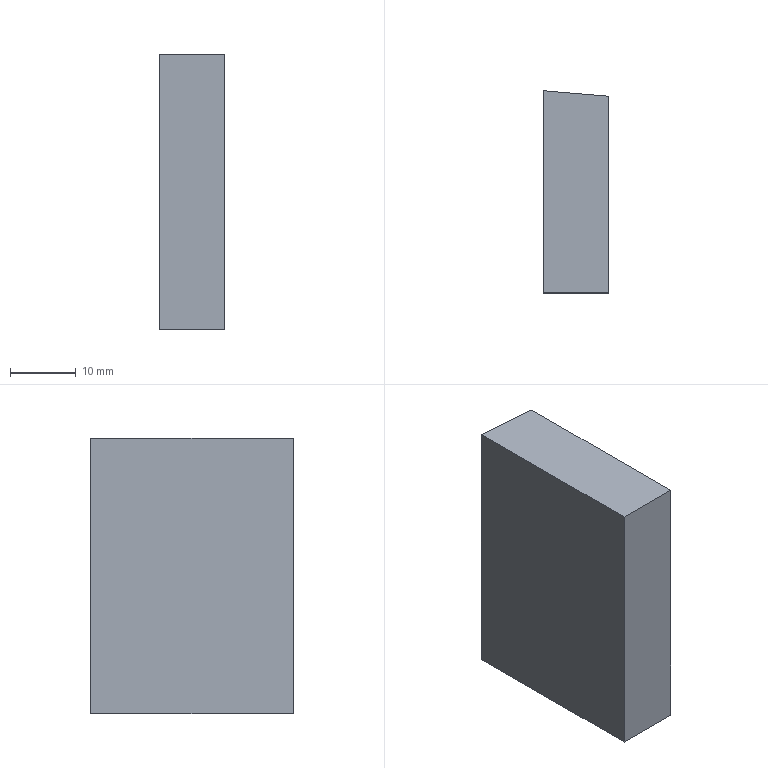Part | SolidWorks | features Extrusion 1 | 1 solid | 6 faces | box 10 x 30.8 x 42 mm | volume 12760 mm3 | plane 6
STEP:
#1=CARTESIAN_POINT('',(0.,30.8,0.));
#2=VERTEX_POINT('',#1);
#3=CARTESIAN_POINT('',(0.,0.,0.));
#4=VERTEX_POINT('',#3);
#5=CARTESIAN_POINT('',(0.,0.,0.));
#6=DIRECTION('',(0.,-1.,0.));
#7=VECTOR('',#6,1000.);
#8=LINE('',#5,#7);
#9=EDGE_CURVE('',#2,#4,#8,.T.);
#10=ORIENTED_EDGE('',*,*,#9,.T.);
#11=CARTESIAN_POINT('',(0.,0.,42.));
#12=VERTEX_POINT('',#11);
#13=CARTESIAN_POINT('',(0.,0.,42.));
#14=DIRECTION('',(0.,0.,-1.));
#15=VECTOR('',#14,1000.);
#16=LINE('',#13,#15);
#17=EDGE_CURVE('',#12,#4,#16,.T.);
#18=ORIENTED_EDGE('',*,*,#17,.F.);
#19=CARTESIAN_POINT('',(0.,30.8,42.));
#20=VERTEX_POINT('',#19);
#21=CARTESIAN_POINT('',(0.,0.,42.));
#22=DIRECTION('',(0.,-1.,0.));
#23=VECTOR('',#22,1000.);
#24=LINE('',#21,#23);
#25=EDGE_CURVE('',#20,#12,#24,.T.);
#26=ORIENTED_EDGE('',*,*,#25,.F.);
#27=CARTESIAN_POINT('',(0.,30.8,42.));
#28=DIRECTION('',(0.,0.,-1.));
#29=VECTOR('',#28,1000.);
#30=LINE('',#27,#29);
#31=EDGE_CURVE('',#20,#2,#30,.T.);
#32=ORIENTED_EDGE('',*,*,#31,.T.);
#33=EDGE_LOOP('',(#10,#18,#26,#32));
#34=FACE_OUTER_BOUND('',#33,.T.);
#35=CARTESIAN_POINT('',(0.,0.,42.));
#36=DIRECTION('',(1.,0.,0.));
#37=DIRECTION('',(0.,0.,-1.));
#38=AXIS2_PLACEMENT_3D('',#35,#36,#37);
#39=PLANE('',#38);
#40=ADVANCED_FACE('',(#34),#39,.F.);
#41=CARTESIAN_POINT('',(10.,0.,0.));
#42=VERTEX_POINT('',#41);
#43=CARTESIAN_POINT('',(0.,0.,0.));
#44=DIRECTION('',(1.,0.,0.));
#45=VECTOR('',#44,1000.);
#46=LINE('',#43,#45);
#47=EDGE_CURVE('',#4,#42,#46,.T.);
#48=ORIENTED_EDGE('',*,*,#47,.T.);
#49=CARTESIAN_POINT('',(10.,0.,42.));
#50=VERTEX_POINT('',#49);
#51=CARTESIAN_POINT('',(10.,0.,42.));
#52=DIRECTION('',(0.,0.,-1.));
#53=VECTOR('',#52,1000.);
#54=LINE('',#51,#53);
#55=EDGE_CURVE('',#50,#42,#54,.T.);
#56=ORIENTED_EDGE('',*,*,#55,.F.);
#57=CARTESIAN_POINT('',(0.,0.,42.));
#58=DIRECTION('',(1.,0.,0.));
#59=VECTOR('',#58,1000.);
#60=LINE('',#57,#59);
#61=EDGE_CURVE('',#12,#50,#60,.T.);
#62=ORIENTED_EDGE('',*,*,#61,.F.);
#63=ORIENTED_EDGE('',*,*,#17,.T.);
#64=EDGE_LOOP('',(#48,#56,#62,#63));
#65=FACE_OUTER_BOUND('',#64,.T.);
#66=CARTESIAN_POINT('',(0.,0.,42.));
#67=DIRECTION('',(0.,1.,0.));
#68=DIRECTION('',(0.,0.,1.));
#69=AXIS2_PLACEMENT_3D('',#66,#67,#68);
#70=PLANE('',#69);
#71=ADVANCED_FACE('',(#65),#70,.F.);
#72=CARTESIAN_POINT('',(10.,29.96,0.));
#73=VERTEX_POINT('',#72);
#74=CARTESIAN_POINT('',(10.,0.,0.));
#75=DIRECTION('',(0.,1.,0.));
#76=VECTOR('',#75,1000.);
#77=LINE('',#74,#76);
#78=EDGE_CURVE('',#42,#73,#77,.T.);
#79=ORIENTED_EDGE('',*,*,#78,.T.);
#80=CARTESIAN_POINT('',(10.,29.96,42.));
#81=VERTEX_POINT('',#80);
#82=CARTESIAN_POINT('',(10.,29.96,42.));
#83=DIRECTION('',(0.,0.,-1.));
#84=VECTOR('',#83,1000.);
#85=LINE('',#82,#84);
#86=EDGE_CURVE('',#81,#73,#85,.T.);
#87=ORIENTED_EDGE('',*,*,#86,.F.);
#88=CARTESIAN_POINT('',(10.,0.,42.));
#89=DIRECTION('',(0.,1.,0.));
#90=VECTOR('',#89,1000.);
#91=LINE('',#88,#90);
#92=EDGE_CURVE('',#50,#81,#91,.T.);
#93=ORIENTED_EDGE('',*,*,#92,.F.);
#94=ORIENTED_EDGE('',*,*,#55,.T.);
#95=EDGE_LOOP('',(#79,#87,#93,#94));
#96=FACE_OUTER_BOUND('',#95,.T.);
#97=CARTESIAN_POINT('',(10.,0.,42.));
#98=DIRECTION('',(-1.,0.,0.));
#99=DIRECTION('',(0.,0.,1.));
#100=AXIS2_PLACEMENT_3D('',#97,#98,#99);
#101=PLANE('',#100);
#102=ADVANCED_FACE('',(#96),#101,.F.);
#103=CARTESIAN_POINT('',(0.,30.8,0.));
#104=DIRECTION('',(-0.9965,0.08368,0.));
#105=VECTOR('',#104,1000.);
#106=LINE('',#103,#105);
#107=EDGE_CURVE('',#73,#2,#106,.T.);
#108=ORIENTED_EDGE('',*,*,#107,.T.);
#109=ORIENTED_EDGE('',*,*,#31,.F.);
#110=CARTESIAN_POINT('',(0.,30.8,42.));
#111=DIRECTION('',(-0.9965,0.08368,0.));
#112=VECTOR('',#111,1000.);
#113=LINE('',#110,#112);
#114=EDGE_CURVE('',#81,#20,#113,.T.);
#115=ORIENTED_EDGE('',*,*,#114,.F.);
#116=ORIENTED_EDGE('',*,*,#86,.T.);
#117=EDGE_LOOP('',(#108,#109,#115,#116));
#118=FACE_OUTER_BOUND('',#117,.T.);
#119=CARTESIAN_POINT('',(0.,30.8,42.));
#120=DIRECTION('',(-0.08368,-0.9965,0.));
#121=DIRECTION('',(0.9965,-0.08368,0.));
#122=AXIS2_PLACEMENT_3D('',#119,#120,#121);
#123=PLANE('',#122);
#124=ADVANCED_FACE('',(#118),#123,.F.);
#125=ORIENTED_EDGE('',*,*,#25,.T.);
#126=ORIENTED_EDGE('',*,*,#61,.T.);
#127=ORIENTED_EDGE('',*,*,#92,.T.);
#128=ORIENTED_EDGE('',*,*,#114,.T.);
#129=EDGE_LOOP('',(#125,#126,#127,#128));
#130=FACE_OUTER_BOUND('',#129,.T.);
#131=CARTESIAN_POINT('',(0.,0.,42.));
#132=DIRECTION('',(0.,0.,-1.));
#133=DIRECTION('',(-1.,0.,0.));
#134=AXIS2_PLACEMENT_3D('',#131,#132,#133);
#135=PLANE('',#134);
#136=ADVANCED_FACE('',(#130),#135,.F.);
#137=ORIENTED_EDGE('',*,*,#9,.F.);
#138=ORIENTED_EDGE('',*,*,#107,.F.);
#139=ORIENTED_EDGE('',*,*,#78,.F.);
#140=ORIENTED_EDGE('',*,*,#47,.F.);
#141=EDGE_LOOP('',(#137,#138,#139,#140));
#142=FACE_OUTER_BOUND('',#141,.T.);
#143=CARTESIAN_POINT('',(0.,0.,0.));
#144=DIRECTION('',(0.,0.,-1.));
#145=DIRECTION('',(-1.,0.,0.));
#146=AXIS2_PLACEMENT_3D('',#143,#144,#145);
#147=PLANE('',#146);
#148=ADVANCED_FACE('',(#142),#147,.T.);
#149=CLOSED_SHELL('',(#40,#71,#102,#124,#136,#148));
#150=MANIFOLD_SOLID_BREP('',#149);
#151=CARTESIAN_POINT('',(0.,0.,0.));
#152=DIRECTION('',(0.,0.,1.));
#153=DIRECTION('',(1.,0.,0.));
#154=AXIS2_PLACEMENT_3D('',#151,#152,#153);
#155=(LENGTH_UNIT()NAMED_UNIT(*)SI_UNIT(.MILLI.,.METRE.));
#156=UNCERTAINTY_MEASURE_WITH_UNIT(LENGTH_MEASURE(0.00001),#155,'','');
#157=(NAMED_UNIT(*)PLANE_ANGLE_UNIT()SI_UNIT($,.RADIAN.));
#158=(NAMED_UNIT(*)SI_UNIT($,.STERADIAN.)SOLID_ANGLE_UNIT());
#159=(GEOMETRIC_REPRESENTATION_CONTEXT(3)GLOBAL_UNCERTAINTY_ASSIGNED_CONTEXT((#156))GLOBAL_UNIT_ASSIGNED_CONTEXT((#155,#157,#158))REPRESENTATION_CONTEXT('',''));
#160=ADVANCED_BREP_SHAPE_REPRESENTATION('',(#150,#154),#159);